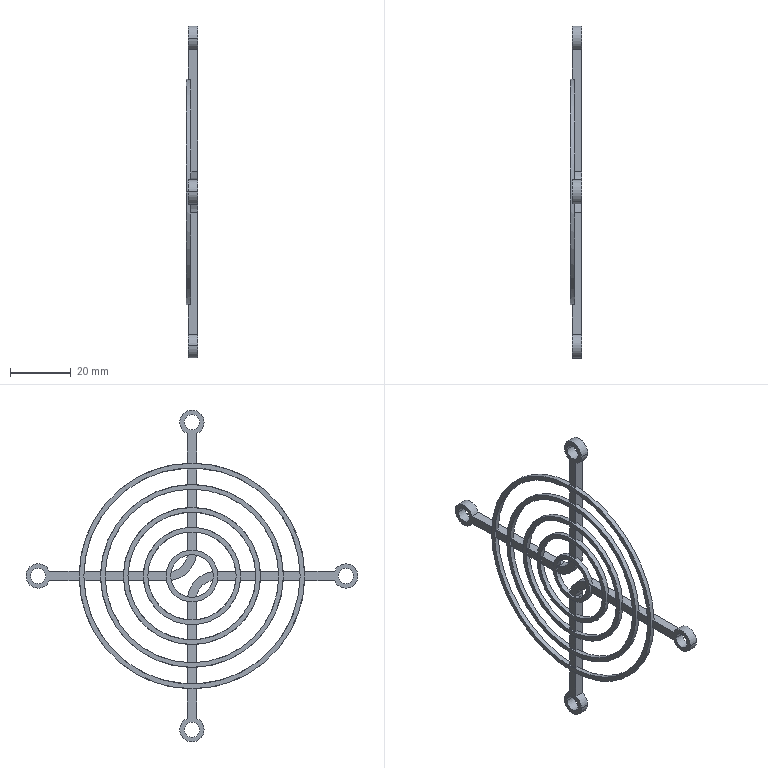Part | STEP file | ZHJ45-80 | 1 solid | 98 faces | box 3.7 x 109.009 x 109.011 mm | volume 3461 mm3 | plane 57 | cylinder 41 | commonest cylinder face diameters 8 x9 5 x8 12.24 x2 14 x2 17 x2 20.206 x2